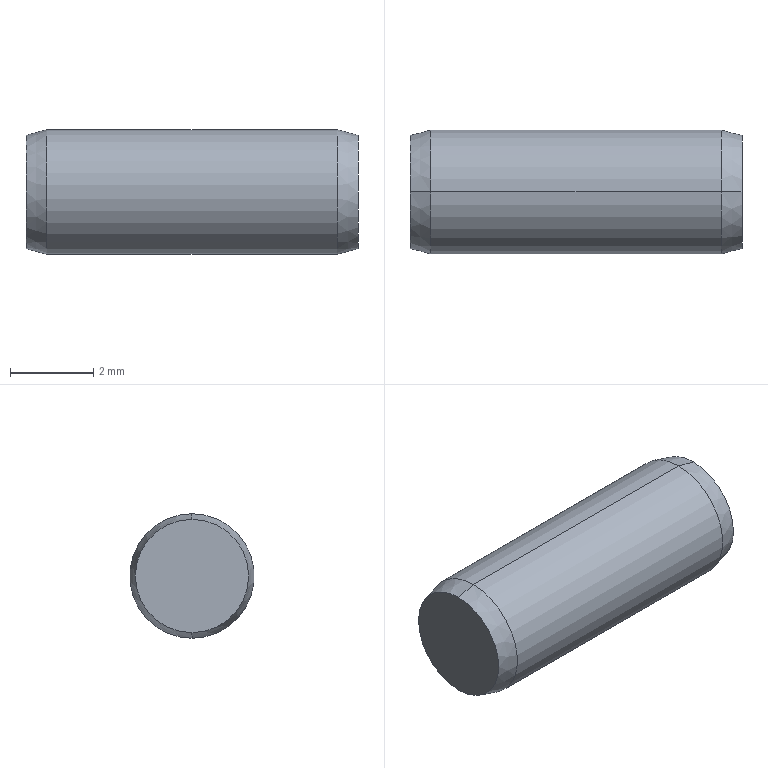Part | NX | features BREP 1 | 1 solid | 8 faces | box 8 x 3 x 3 mm | volume 55.936 mm3 | cone 4 | cylinder 2 | plane 2 | commonest cylinder face diameters 3 x2
STEP:
#1=CARTESIAN_POINT('',(-1.,0.,-1.5));
#2=VERTEX_POINT('',#1);
#3=CARTESIAN_POINT('',(6.,0.,-1.5));
#4=VERTEX_POINT('',#3);
#5=CARTESIAN_POINT('',(0.,0.,-1.5));
#6=DIRECTION('',(-1.,0.,0.));
#7=VECTOR('',#6,1000.);
#8=LINE('',#5,#7);
#9=EDGE_CURVE('',#2,#4,#8,.F.);
#10=ORIENTED_EDGE('',*,*,#9,.T.);
#11=CARTESIAN_POINT('',(6.,0.,1.5));
#12=VERTEX_POINT('',#11);
#13=CARTESIAN_POINT('',(6.,0.,0.));
#14=DIRECTION('',(-1.,0.,0.));
#15=DIRECTION('',(0.,0.,1.));
#16=AXIS2_PLACEMENT_3D('',#13,#14,#15);
#17=CIRCLE('',#16,1.5);
#18=EDGE_CURVE('',#4,#12,#17,.T.);
#19=ORIENTED_EDGE('',*,*,#18,.T.);
#20=CARTESIAN_POINT('',(-1.,0.,1.5));
#21=VERTEX_POINT('',#20);
#22=CARTESIAN_POINT('',(0.,0.,1.5));
#23=DIRECTION('',(-1.,0.,0.));
#24=VECTOR('',#23,1000.);
#25=LINE('',#22,#24);
#26=EDGE_CURVE('',#21,#12,#25,.F.);
#27=ORIENTED_EDGE('',*,*,#26,.F.);
#28=CARTESIAN_POINT('',(-1.,0.,0.));
#29=DIRECTION('',(-1.,0.,0.));
#30=DIRECTION('',(0.,0.,1.));
#31=AXIS2_PLACEMENT_3D('',#28,#29,#30);
#32=CIRCLE('',#31,1.5);
#33=EDGE_CURVE('',#2,#21,#32,.T.);
#34=ORIENTED_EDGE('',*,*,#33,.F.);
#35=EDGE_LOOP('',(#10,#19,#27,#34));
#36=FACE_BOUND('',#35,.T.);
#37=CARTESIAN_POINT('',(0.,0.,0.));
#38=DIRECTION('',(-1.,0.,0.));
#39=DIRECTION('',(0.,0.,1.));
#40=AXIS2_PLACEMENT_3D('',#37,#38,#39);
#41=CYLINDRICAL_SURFACE('',#40,1.5);
#42=ADVANCED_FACE('',(#36),#41,.T.);
#43=CARTESIAN_POINT('',(-1.5,0.,1.366));
#44=VERTEX_POINT('',#43);
#45=CARTESIAN_POINT('',(-1.,0.,1.5));
#46=DIRECTION('',(0.9659,0.,0.2588));
#47=VECTOR('',#46,1000.);
#48=LINE('',#45,#47);
#49=EDGE_CURVE('',#44,#21,#48,.T.);
#50=ORIENTED_EDGE('',*,*,#49,.F.);
#51=CARTESIAN_POINT('',(-1.5,0.,-1.366));
#52=VERTEX_POINT('',#51);
#53=CARTESIAN_POINT('',(-1.5,0.,0.));
#54=DIRECTION('',(-1.,0.,0.));
#55=DIRECTION('',(0.,0.,1.));
#56=AXIS2_PLACEMENT_3D('',#53,#54,#55);
#57=CIRCLE('',#56,1.366);
#58=EDGE_CURVE('',#52,#44,#57,.T.);
#59=ORIENTED_EDGE('',*,*,#58,.F.);
#60=CARTESIAN_POINT('',(-1.,0.,-1.5));
#61=DIRECTION('',(0.9659,0.,-0.2588));
#62=VECTOR('',#61,1000.);
#63=LINE('',#60,#62);
#64=EDGE_CURVE('',#52,#2,#63,.T.);
#65=ORIENTED_EDGE('',*,*,#64,.T.);
#66=ORIENTED_EDGE('',*,*,#33,.T.);
#67=EDGE_LOOP('',(#50,#59,#65,#66));
#68=FACE_BOUND('',#67,.T.);
#69=CARTESIAN_POINT('',(-1.,0.,0.));
#70=DIRECTION('',(1.,0.,0.));
#71=DIRECTION('',(0.,0.,-1.));
#72=AXIS2_PLACEMENT_3D('',#69,#70,#71);
#73=CONICAL_SURFACE('',#72,1.5,0.2618);
#74=ADVANCED_FACE('',(#68),#73,.T.);
#75=ORIENTED_EDGE('',*,*,#58,.T.);
#76=CARTESIAN_POINT('',(-1.5,0.,0.));
#77=DIRECTION('',(-1.,0.,0.));
#78=DIRECTION('',(0.,0.,1.));
#79=AXIS2_PLACEMENT_3D('',#76,#77,#78);
#80=CIRCLE('',#79,1.366);
#81=EDGE_CURVE('',#44,#52,#80,.T.);
#82=ORIENTED_EDGE('',*,*,#81,.T.);
#83=EDGE_LOOP('',(#75,#82));
#84=FACE_BOUND('',#83,.T.);
#85=CARTESIAN_POINT('',(-1.5,1.366,0.));
#86=DIRECTION('',(1.,0.,0.));
#87=DIRECTION('',(0.,0.,-1.));
#88=AXIS2_PLACEMENT_3D('',#85,#86,#87);
#89=PLANE('',#88);
#90=ADVANCED_FACE('',(#84),#89,.F.);
#91=CARTESIAN_POINT('',(6.5,0.,1.366));
#92=VERTEX_POINT('',#91);
#93=CARTESIAN_POINT('',(6.5,0.,-1.366));
#94=VERTEX_POINT('',#93);
#95=CARTESIAN_POINT('',(6.5,0.,0.));
#96=DIRECTION('',(-1.,0.,0.));
#97=DIRECTION('',(0.,0.,1.));
#98=AXIS2_PLACEMENT_3D('',#95,#96,#97);
#99=CIRCLE('',#98,1.366);
#100=EDGE_CURVE('',#92,#94,#99,.T.);
#101=ORIENTED_EDGE('',*,*,#100,.F.);
#102=CARTESIAN_POINT('',(6.5,0.,0.));
#103=DIRECTION('',(-1.,0.,0.));
#104=DIRECTION('',(0.,0.,1.));
#105=AXIS2_PLACEMENT_3D('',#102,#103,#104);
#106=CIRCLE('',#105,1.366);
#107=EDGE_CURVE('',#94,#92,#106,.T.);
#108=ORIENTED_EDGE('',*,*,#107,.F.);
#109=EDGE_LOOP('',(#101,#108));
#110=FACE_BOUND('',#109,.T.);
#111=CARTESIAN_POINT('',(6.5,1.366,0.));
#112=DIRECTION('',(-1.,0.,0.));
#113=DIRECTION('',(0.,0.,1.));
#114=AXIS2_PLACEMENT_3D('',#111,#112,#113);
#115=PLANE('',#114);
#116=ADVANCED_FACE('',(#110),#115,.F.);
#117=CARTESIAN_POINT('',(6.5,0.,-1.366));
#118=DIRECTION('',(-0.9659,0.,-0.2588));
#119=VECTOR('',#118,1000.);
#120=LINE('',#117,#119);
#121=EDGE_CURVE('',#4,#94,#120,.F.);
#122=ORIENTED_EDGE('',*,*,#121,.T.);
#123=ORIENTED_EDGE('',*,*,#107,.T.);
#124=CARTESIAN_POINT('',(6.5,0.,1.366));
#125=DIRECTION('',(-0.9659,0.,0.2588));
#126=VECTOR('',#125,1000.);
#127=LINE('',#124,#126);
#128=EDGE_CURVE('',#12,#92,#127,.F.);
#129=ORIENTED_EDGE('',*,*,#128,.F.);
#130=ORIENTED_EDGE('',*,*,#18,.F.);
#131=EDGE_LOOP('',(#122,#123,#129,#130));
#132=FACE_BOUND('',#131,.T.);
#133=CARTESIAN_POINT('',(6.5,0.,0.));
#134=DIRECTION('',(-1.,0.,0.));
#135=DIRECTION('',(0.,0.,1.));
#136=AXIS2_PLACEMENT_3D('',#133,#134,#135);
#137=CONICAL_SURFACE('',#136,1.366,0.2618);
#138=ADVANCED_FACE('',(#132),#137,.T.);
#139=ORIENTED_EDGE('',*,*,#100,.T.);
#140=ORIENTED_EDGE('',*,*,#121,.F.);
#141=CARTESIAN_POINT('',(6.,0.,0.));
#142=DIRECTION('',(-1.,0.,0.));
#143=DIRECTION('',(0.,0.,1.));
#144=AXIS2_PLACEMENT_3D('',#141,#142,#143);
#145=CIRCLE('',#144,1.5);
#146=EDGE_CURVE('',#12,#4,#145,.T.);
#147=ORIENTED_EDGE('',*,*,#146,.F.);
#148=ORIENTED_EDGE('',*,*,#128,.T.);
#149=EDGE_LOOP('',(#139,#140,#147,#148));
#150=FACE_BOUND('',#149,.T.);
#151=CARTESIAN_POINT('',(6.5,0.,0.));
#152=DIRECTION('',(-1.,0.,0.));
#153=DIRECTION('',(0.,0.,1.));
#154=AXIS2_PLACEMENT_3D('',#151,#152,#153);
#155=CONICAL_SURFACE('',#154,1.366,0.2618);
#156=ADVANCED_FACE('',(#150),#155,.T.);
#157=ORIENTED_EDGE('',*,*,#81,.F.);
#158=ORIENTED_EDGE('',*,*,#49,.T.);
#159=CARTESIAN_POINT('',(-1.,0.,0.));
#160=DIRECTION('',(-1.,0.,0.));
#161=DIRECTION('',(0.,0.,1.));
#162=AXIS2_PLACEMENT_3D('',#159,#160,#161);
#163=CIRCLE('',#162,1.5);
#164=EDGE_CURVE('',#21,#2,#163,.T.);
#165=ORIENTED_EDGE('',*,*,#164,.T.);
#166=ORIENTED_EDGE('',*,*,#64,.F.);
#167=EDGE_LOOP('',(#157,#158,#165,#166));
#168=FACE_BOUND('',#167,.T.);
#169=CARTESIAN_POINT('',(-1.,0.,0.));
#170=DIRECTION('',(1.,0.,0.));
#171=DIRECTION('',(0.,0.,-1.));
#172=AXIS2_PLACEMENT_3D('',#169,#170,#171);
#173=CONICAL_SURFACE('',#172,1.5,0.2618);
#174=ADVANCED_FACE('',(#168),#173,.T.);
#175=ORIENTED_EDGE('',*,*,#146,.T.);
#176=ORIENTED_EDGE('',*,*,#9,.F.);
#177=ORIENTED_EDGE('',*,*,#164,.F.);
#178=ORIENTED_EDGE('',*,*,#26,.T.);
#179=EDGE_LOOP('',(#175,#176,#177,#178));
#180=FACE_BOUND('',#179,.T.);
#181=CARTESIAN_POINT('',(0.,0.,0.));
#182=DIRECTION('',(-1.,0.,0.));
#183=DIRECTION('',(0.,0.,1.));
#184=AXIS2_PLACEMENT_3D('',#181,#182,#183);
#185=CYLINDRICAL_SURFACE('',#184,1.5);
#186=ADVANCED_FACE('',(#180),#185,.T.);
#187=CLOSED_SHELL('',(#42,#74,#90,#116,#138,#156,#174,#186));
#188=MANIFOLD_SOLID_BREP('',#187);
#189=(LENGTH_UNIT()NAMED_UNIT(*)SI_UNIT(.MILLI.,.METRE.));
#190=UNCERTAINTY_MEASURE_WITH_UNIT(LENGTH_MEASURE(0.00001),#189,'','');
#191=(NAMED_UNIT(*)PLANE_ANGLE_UNIT()SI_UNIT($,.RADIAN.));
#192=(NAMED_UNIT(*)SI_UNIT($,.STERADIAN.)SOLID_ANGLE_UNIT());
#193=(GEOMETRIC_REPRESENTATION_CONTEXT(3)GLOBAL_UNCERTAINTY_ASSIGNED_CONTEXT((#190))GLOBAL_UNIT_ASSIGNED_CONTEXT((#189,#191,#192))REPRESENTATION_CONTEXT('',''));
#194=ADVANCED_BREP_SHAPE_REPRESENTATION('',(#188),#193);